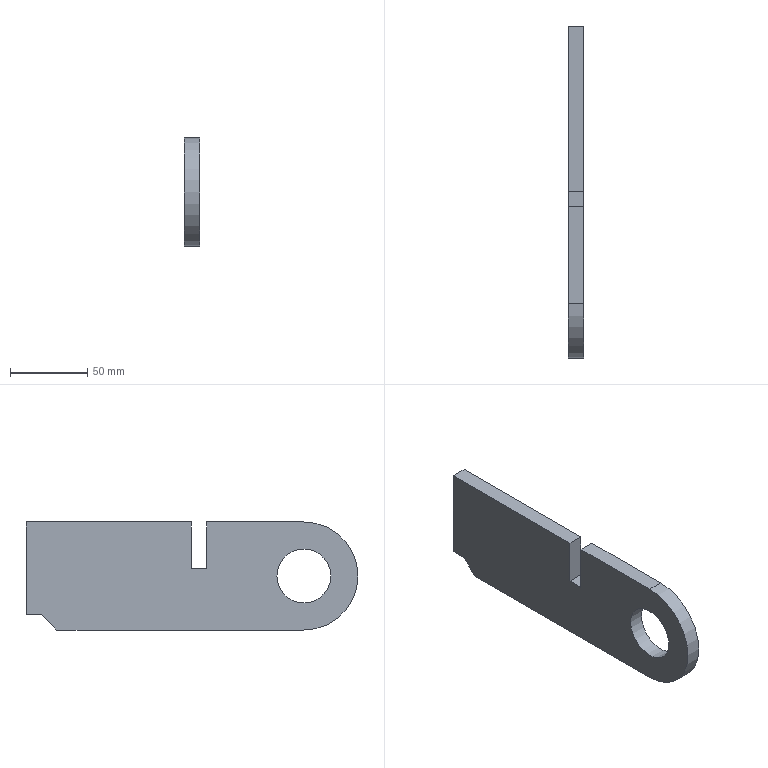Part | STEP file | subframe tilt cylinder mounting plate--000.0
01--20240928 | 1 solid | 13 faces | box 10 x 215 x 70 mm | volume 131121 mm3 | plane 11 | cylinder 2 | commonest cylinder face diameters 35 x1 70 x1
STEP:
#1=CARTESIAN_POINT('',(0.,0.,0.));
#2=DIRECTION('',(0.,0.,1.));
#3=DIRECTION('',(1.,0.,0.));
#4=AXIS2_PLACEMENT_3D('',#1,#2,#3);
#5=CARTESIAN_POINT('',(-630.,216.,-35.));
#6=VERTEX_POINT('',#5);
#7=CARTESIAN_POINT('',(-630.,198.5,-35.));
#8=DIRECTION('',(1.,0.,0.));
#9=DIRECTION('',(0.,1.,0.));
#10=AXIS2_PLACEMENT_3D('',#7,#8,#9);
#11=CIRCLE('',#10,17.5);
#12=CARTESIAN_POINT('',(-630.,-284.,-150.));
#13=DIRECTION('',(1.,0.,0.));
#14=DIRECTION('',(0.,-1.,0.));
#15=AXIS2_PLACEMENT_3D('',#12,#13,#14);
#16=PLANE('',#15);
#17=CARTESIAN_POINT('',(-482.5,-115.));
#18=DIRECTION('',(-1.,0.));
#19=AXIS2_PLACEMENT_2D('',#17,#18);
#20=CIRCLE('',#19,17.5);
#21=(GEOMETRIC_REPRESENTATION_CONTEXT(2)PARAMETRIC_REPRESENTATION_CONTEXT()REPRESENTATION_CONTEXT('',''));
#22=DEFINITIONAL_REPRESENTATION('',(#20),#21);
#23=PCURVE('',#16,#22);
#24=CARTESIAN_POINT('',(-1050.,198.5,-35.));
#25=DIRECTION('',(1.,0.,0.));
#26=DIRECTION('',(0.,0.,1.));
#27=AXIS2_PLACEMENT_3D('',#24,#25,#26);
#28=CYLINDRICAL_SURFACE('',#27,17.5);
#29=CARTESIAN_POINT('',(4.712,420.));
#30=DIRECTION('',(1.,0.));
#31=VECTOR('',#30,1.);
#32=LINE('',#29,#31);
#33=(GEOMETRIC_REPRESENTATION_CONTEXT(2)PARAMETRIC_REPRESENTATION_CONTEXT()REPRESENTATION_CONTEXT('',''));
#34=DEFINITIONAL_REPRESENTATION('',(#32),#33);
#35=PCURVE('',#28,#34);
#36=SURFACE_CURVE('',#11,(#23,#35),.PCURVE_S1.);
#37=EDGE_CURVE('',#6,#6,#36,.T.);
#38=ORIENTED_EDGE('',*,*,#37,.F.);
#39=EDGE_LOOP('',(#38));
#40=FACE_BOUND('',#39,.T.);
#41=CARTESIAN_POINT('',(-630.,198.5,0.));
#42=VERTEX_POINT('',#41);
#43=CARTESIAN_POINT('',(-630.,198.5,-70.));
#44=VERTEX_POINT('',#43);
#45=CARTESIAN_POINT('',(-630.,198.5,-35.));
#46=DIRECTION('',(1.,0.,0.));
#47=DIRECTION('',(0.,1.,0.));
#48=AXIS2_PLACEMENT_3D('',#45,#46,#47);
#49=CIRCLE('',#48,35.);
#50=CARTESIAN_POINT('',(-482.5,-115.));
#51=DIRECTION('',(-1.,0.));
#52=AXIS2_PLACEMENT_2D('',#50,#51);
#53=CIRCLE('',#52,35.);
#54=(GEOMETRIC_REPRESENTATION_CONTEXT(2)PARAMETRIC_REPRESENTATION_CONTEXT()REPRESENTATION_CONTEXT('',''));
#55=DEFINITIONAL_REPRESENTATION('',(#53),#54);
#56=PCURVE('',#16,#55);
#57=CARTESIAN_POINT('',(-700.,198.5,-35.));
#58=DIRECTION('',(-1.,0.,0.));
#59=DIRECTION('',(0.,0.,-1.));
#60=AXIS2_PLACEMENT_3D('',#57,#58,#59);
#61=CYLINDRICAL_SURFACE('',#60,35.);
#62=CARTESIAN_POINT('',(4.712,-70.));
#63=DIRECTION('',(-1.,0.));
#64=VECTOR('',#63,1.);
#65=LINE('',#62,#64);
#66=(GEOMETRIC_REPRESENTATION_CONTEXT(2)PARAMETRIC_REPRESENTATION_CONTEXT()REPRESENTATION_CONTEXT('',''));
#67=DEFINITIONAL_REPRESENTATION('',(#65),#66);
#68=PCURVE('',#61,#67);
#69=SURFACE_CURVE('',#49,(#56,#68),.PCURVE_S1.);
#70=EDGE_CURVE('',#42,#44,#69,.T.);
#71=ORIENTED_EDGE('',*,*,#70,.T.);
#72=CARTESIAN_POINT('',(-630.,358.5,-70.));
#73=VERTEX_POINT('',#72);
#74=CARTESIAN_POINT('',(-630.,198.5,-70.));
#75=DIRECTION('',(0.,-1.,0.));
#76=VECTOR('',#75,1.);
#77=LINE('',#74,#76);
#78=CARTESIAN_POINT('',(-482.5,-80.));
#79=DIRECTION('',(1.,0.));
#80=VECTOR('',#79,1.);
#81=LINE('',#78,#80);
#82=(GEOMETRIC_REPRESENTATION_CONTEXT(2)PARAMETRIC_REPRESENTATION_CONTEXT()REPRESENTATION_CONTEXT('',''));
#83=DEFINITIONAL_REPRESENTATION('',(#81),#82);
#84=PCURVE('',#16,#83);
#85=CARTESIAN_POINT('',(-700.,198.5,-70.));
#86=DIRECTION('',(0.,0.,-1.));
#87=DIRECTION('',(1.,0.,0.));
#88=AXIS2_PLACEMENT_3D('',#85,#86,#87);
#89=PLANE('',#88);
#90=CARTESIAN_POINT('',(70.,0.));
#91=DIRECTION('',(0.,1.));
#92=VECTOR('',#91,1.);
#93=LINE('',#90,#92);
#94=(GEOMETRIC_REPRESENTATION_CONTEXT(2)PARAMETRIC_REPRESENTATION_CONTEXT()REPRESENTATION_CONTEXT('',''));
#95=DEFINITIONAL_REPRESENTATION('',(#93),#94);
#96=PCURVE('',#89,#95);
#97=SURFACE_CURVE('',#77,(#84,#96),.PCURVE_S1.);
#98=EDGE_CURVE('',#73,#44,#97,.T.);
#99=ORIENTED_EDGE('',*,*,#98,.F.);
#100=CARTESIAN_POINT('',(-630.,368.5,-60.));
#101=VERTEX_POINT('',#100);
#102=CARTESIAN_POINT('',(-630.,-2.75,-431.25));
#103=DIRECTION('',(0.,0.7071,0.7071));
#104=VECTOR('',#103,1.);
#105=LINE('',#102,#104);
#106=CARTESIAN_POINT('',(-281.25,281.25));
#107=DIRECTION('',(-0.7071,-0.7071));
#108=VECTOR('',#107,1.);
#109=LINE('',#106,#108);
#110=(GEOMETRIC_REPRESENTATION_CONTEXT(2)PARAMETRIC_REPRESENTATION_CONTEXT()REPRESENTATION_CONTEXT('',''));
#111=DEFINITIONAL_REPRESENTATION('',(#109),#110);
#112=PCURVE('',#16,#111);
#113=CARTESIAN_POINT('',(600.173,368.5,-60.));
#114=DIRECTION('',(0.,-0.7071,0.7071));
#115=DIRECTION('',(1.,0.,0.));
#116=AXIS2_PLACEMENT_3D('',#113,#114,#115);
#117=PLANE('',#116);
#118=CARTESIAN_POINT('',(-1230.173,-525.027));
#119=DIRECTION('',(0.,1.));
#120=VECTOR('',#119,1.);
#121=LINE('',#118,#120);
#122=(GEOMETRIC_REPRESENTATION_CONTEXT(2)PARAMETRIC_REPRESENTATION_CONTEXT()REPRESENTATION_CONTEXT('',''));
#123=DEFINITIONAL_REPRESENTATION('',(#121),#122);
#124=PCURVE('',#117,#123);
#125=SURFACE_CURVE('',#105,(#112,#124),.PCURVE_S1.);
#126=EDGE_CURVE('',#73,#101,#125,.T.);
#127=ORIENTED_EDGE('',*,*,#126,.T.);
#128=CARTESIAN_POINT('',(-630.,378.5,-60.));
#129=VERTEX_POINT('',#128);
#130=CARTESIAN_POINT('',(-630.,-284.,-60.));
#131=DIRECTION('',(0.,1.,0.));
#132=VECTOR('',#131,1.);
#133=LINE('',#130,#132);
#134=CARTESIAN_POINT('',(0.,-90.));
#135=DIRECTION('',(-1.,0.));
#136=VECTOR('',#135,1.);
#137=LINE('',#134,#136);
#138=(GEOMETRIC_REPRESENTATION_CONTEXT(2)PARAMETRIC_REPRESENTATION_CONTEXT()REPRESENTATION_CONTEXT('',''));
#139=DEFINITIONAL_REPRESENTATION('',(#137),#138);
#140=PCURVE('',#16,#139);
#141=CARTESIAN_POINT('',(-635.,288.5,-60.));
#142=DIRECTION('',(0.,0.,-1.));
#143=DIRECTION('',(1.,0.,0.));
#144=AXIS2_PLACEMENT_3D('',#141,#142,#143);
#145=PLANE('',#144);
#146=CARTESIAN_POINT('',(5.,572.5));
#147=DIRECTION('',(0.,-1.));
#148=VECTOR('',#147,1.);
#149=LINE('',#146,#148);
#150=(GEOMETRIC_REPRESENTATION_CONTEXT(2)PARAMETRIC_REPRESENTATION_CONTEXT()REPRESENTATION_CONTEXT('',''));
#151=DEFINITIONAL_REPRESENTATION('',(#149),#150);
#152=PCURVE('',#145,#151);
#153=SURFACE_CURVE('',#133,(#140,#152),.PCURVE_S1.);
#154=EDGE_CURVE('',#101,#129,#153,.T.);
#155=ORIENTED_EDGE('',*,*,#154,.T.);
#156=CARTESIAN_POINT('',(-630.,378.5,0.));
#157=VERTEX_POINT('',#156);
#158=CARTESIAN_POINT('',(-630.,378.5,-20.));
#159=DIRECTION('',(0.,0.,-1.));
#160=VECTOR('',#159,1.);
#161=LINE('',#158,#160);
#162=CARTESIAN_POINT('',(-662.5,-130.));
#163=DIRECTION('',(0.,1.));
#164=VECTOR('',#163,1.);
#165=LINE('',#162,#164);
#166=(GEOMETRIC_REPRESENTATION_CONTEXT(2)PARAMETRIC_REPRESENTATION_CONTEXT()REPRESENTATION_CONTEXT('',''));
#167=DEFINITIONAL_REPRESENTATION('',(#165),#166);
#168=PCURVE('',#16,#167);
#169=CARTESIAN_POINT('',(600.173,378.5,-20.));
#170=DIRECTION('',(0.,1.,0.));
#171=DIRECTION('',(0.9613,0.,0.2756));
#172=AXIS2_PLACEMENT_3D('',#169,#170,#171);
#173=PLANE('',#172);
#174=CARTESIAN_POINT('',(-1182.518,-339.082));
#175=DIRECTION('',(-0.2756,0.9613));
#176=VECTOR('',#175,1.);
#177=LINE('',#174,#176);
#178=(GEOMETRIC_REPRESENTATION_CONTEXT(2)PARAMETRIC_REPRESENTATION_CONTEXT()REPRESENTATION_CONTEXT('',''));
#179=DEFINITIONAL_REPRESENTATION('',(#177),#178);
#180=PCURVE('',#173,#179);
#181=SURFACE_CURVE('',#161,(#168,#180),.PCURVE_S1.);
#182=EDGE_CURVE('',#157,#129,#181,.T.);
#183=ORIENTED_EDGE('',*,*,#182,.F.);
#184=CARTESIAN_POINT('',(-630.,271.5,0.));
#185=VERTEX_POINT('',#184);
#186=CARTESIAN_POINT('',(-630.,-488.,0.));
#187=DIRECTION('',(0.,1.,0.));
#188=VECTOR('',#187,1.);
#189=LINE('',#186,#188);
#190=CARTESIAN_POINT('',(204.,-150.));
#191=DIRECTION('',(-1.,0.));
#192=VECTOR('',#191,1.);
#193=LINE('',#190,#192);
#194=(GEOMETRIC_REPRESENTATION_CONTEXT(2)PARAMETRIC_REPRESENTATION_CONTEXT()REPRESENTATION_CONTEXT('',''));
#195=DEFINITIONAL_REPRESENTATION('',(#193),#194);
#196=PCURVE('',#16,#195);
#197=CARTESIAN_POINT('',(-750.,-488.,0.));
#198=DIRECTION('',(0.,0.,1.));
#199=DIRECTION('',(0.,1.,0.));
#200=AXIS2_PLACEMENT_3D('',#197,#198,#199);
#201=PLANE('',#200);
#202=CARTESIAN_POINT('',(0.,-120.));
#203=DIRECTION('',(1.,0.));
#204=VECTOR('',#203,1.);
#205=LINE('',#202,#204);
#206=(GEOMETRIC_REPRESENTATION_CONTEXT(2)PARAMETRIC_REPRESENTATION_CONTEXT()REPRESENTATION_CONTEXT('',''));
#207=DEFINITIONAL_REPRESENTATION('',(#205),#206);
#208=PCURVE('',#201,#207);
#209=SURFACE_CURVE('',#189,(#196,#208),.PCURVE_S1.);
#210=EDGE_CURVE('',#185,#157,#209,.T.);
#211=ORIENTED_EDGE('',*,*,#210,.F.);
#212=CARTESIAN_POINT('',(-630.,271.5,-30.));
#213=VERTEX_POINT('',#212);
#214=CARTESIAN_POINT('',(-630.,271.5,-150.));
#215=DIRECTION('',(0.,0.,1.));
#216=VECTOR('',#215,1.);
#217=LINE('',#214,#216);
#218=CARTESIAN_POINT('',(-555.5,0.));
#219=DIRECTION('',(0.,-1.));
#220=VECTOR('',#219,1.);
#221=LINE('',#218,#220);
#222=(GEOMETRIC_REPRESENTATION_CONTEXT(2)PARAMETRIC_REPRESENTATION_CONTEXT()REPRESENTATION_CONTEXT('',''));
#223=DEFINITIONAL_REPRESENTATION('',(#221),#222);
#224=PCURVE('',#16,#223);
#225=CARTESIAN_POINT('',(-630.,271.5,-60.));
#226=DIRECTION('',(0.,1.,0.));
#227=DIRECTION('',(0.,0.,-1.));
#228=AXIS2_PLACEMENT_3D('',#225,#226,#227);
#229=PLANE('',#228);
#230=CARTESIAN_POINT('',(90.,0.));
#231=DIRECTION('',(-1.,0.));
#232=VECTOR('',#231,1.);
#233=LINE('',#230,#232);
#234=(GEOMETRIC_REPRESENTATION_CONTEXT(2)PARAMETRIC_REPRESENTATION_CONTEXT()REPRESENTATION_CONTEXT('',''));
#235=DEFINITIONAL_REPRESENTATION('',(#233),#234);
#236=PCURVE('',#229,#235);
#237=SURFACE_CURVE('',#217,(#224,#236),.PCURVE_S1.);
#238=EDGE_CURVE('',#213,#185,#237,.T.);
#239=ORIENTED_EDGE('',*,*,#238,.F.);
#240=CARTESIAN_POINT('',(-630.,261.5,-30.));
#241=VERTEX_POINT('',#240);
#242=CARTESIAN_POINT('',(-630.,266.5,-30.));
#243=DIRECTION('',(0.,1.,0.));
#244=VECTOR('',#243,1.);
#245=LINE('',#242,#244);
#246=CARTESIAN_POINT('',(-550.5,-120.));
#247=DIRECTION('',(-1.,0.));
#248=VECTOR('',#247,1.);
#249=LINE('',#246,#248);
#250=(GEOMETRIC_REPRESENTATION_CONTEXT(2)PARAMETRIC_REPRESENTATION_CONTEXT()REPRESENTATION_CONTEXT('',''));
#251=DEFINITIONAL_REPRESENTATION('',(#249),#250);
#252=PCURVE('',#16,#251);
#253=CARTESIAN_POINT('',(-625.,266.5,-30.));
#254=DIRECTION('',(0.,0.,1.));
#255=DIRECTION('',(-1.,0.,0.));
#256=AXIS2_PLACEMENT_3D('',#253,#254,#255);
#257=PLANE('',#256);
#258=CARTESIAN_POINT('',(5.,0.));
#259=DIRECTION('',(0.,-1.));
#260=VECTOR('',#259,1.);
#261=LINE('',#258,#260);
#262=(GEOMETRIC_REPRESENTATION_CONTEXT(2)PARAMETRIC_REPRESENTATION_CONTEXT()REPRESENTATION_CONTEXT('',''));
#263=DEFINITIONAL_REPRESENTATION('',(#261),#262);
#264=PCURVE('',#257,#263);
#265=SURFACE_CURVE('',#245,(#252,#264),.PCURVE_S1.);
#266=EDGE_CURVE('',#241,#213,#265,.T.);
#267=ORIENTED_EDGE('',*,*,#266,.F.);
#268=CARTESIAN_POINT('',(-630.,261.5,0.));
#269=VERTEX_POINT('',#268);
#270=CARTESIAN_POINT('',(-630.,261.5,-150.));
#271=DIRECTION('',(0.,0.,-1.));
#272=VECTOR('',#271,1.);
#273=LINE('',#270,#272);
#274=CARTESIAN_POINT('',(-545.5,0.));
#275=DIRECTION('',(0.,1.));
#276=VECTOR('',#275,1.);
#277=LINE('',#274,#276);
#278=(GEOMETRIC_REPRESENTATION_CONTEXT(2)PARAMETRIC_REPRESENTATION_CONTEXT()REPRESENTATION_CONTEXT('',''));
#279=DEFINITIONAL_REPRESENTATION('',(#277),#278);
#280=PCURVE('',#16,#279);
#281=CARTESIAN_POINT('',(-630.,261.5,-60.));
#282=DIRECTION('',(0.,1.,0.));
#283=DIRECTION('',(0.,0.,-1.));
#284=AXIS2_PLACEMENT_3D('',#281,#282,#283);
#285=PLANE('',#284);
#286=CARTESIAN_POINT('',(90.,0.));
#287=DIRECTION('',(1.,0.));
#288=VECTOR('',#287,1.);
#289=LINE('',#286,#288);
#290=(GEOMETRIC_REPRESENTATION_CONTEXT(2)PARAMETRIC_REPRESENTATION_CONTEXT()REPRESENTATION_CONTEXT('',''));
#291=DEFINITIONAL_REPRESENTATION('',(#289),#290);
#292=PCURVE('',#285,#291);
#293=SURFACE_CURVE('',#273,(#280,#292),.PCURVE_S1.);
#294=EDGE_CURVE('',#269,#241,#293,.T.);
#295=ORIENTED_EDGE('',*,*,#294,.F.);
#296=CARTESIAN_POINT('',(-630.,-488.,0.));
#297=DIRECTION('',(0.,1.,0.));
#298=VECTOR('',#297,1.);
#299=LINE('',#296,#298);
#300=CARTESIAN_POINT('',(204.,-150.));
#301=DIRECTION('',(-1.,0.));
#302=VECTOR('',#301,1.);
#303=LINE('',#300,#302);
#304=(GEOMETRIC_REPRESENTATION_CONTEXT(2)PARAMETRIC_REPRESENTATION_CONTEXT()REPRESENTATION_CONTEXT('',''));
#305=DEFINITIONAL_REPRESENTATION('',(#303),#304);
#306=PCURVE('',#16,#305);
#307=CARTESIAN_POINT('',(-750.,-488.,0.));
#308=DIRECTION('',(0.,0.,1.));
#309=DIRECTION('',(0.,1.,0.));
#310=AXIS2_PLACEMENT_3D('',#307,#308,#309);
#311=PLANE('',#310);
#312=CARTESIAN_POINT('',(0.,-120.));
#313=DIRECTION('',(1.,0.));
#314=VECTOR('',#313,1.);
#315=LINE('',#312,#314);
#316=(GEOMETRIC_REPRESENTATION_CONTEXT(2)PARAMETRIC_REPRESENTATION_CONTEXT()REPRESENTATION_CONTEXT('',''));
#317=DEFINITIONAL_REPRESENTATION('',(#315),#316);
#318=PCURVE('',#311,#317);
#319=SURFACE_CURVE('',#299,(#306,#318),.PCURVE_S1.);
#320=EDGE_CURVE('',#42,#269,#319,.T.);
#321=ORIENTED_EDGE('',*,*,#320,.F.);
#322=EDGE_LOOP('',(#71,#99,#127,#155,#183,#211,#239,#267,#295,#321));
#323=FACE_BOUND('',#322,.T.);
#324=ADVANCED_FACE('',(#40,#323),#16,.T.);
#325=CARTESIAN_POINT('',(-640.,181.,-35.));
#326=VERTEX_POINT('',#325);
#327=CARTESIAN_POINT('',(-640.,216.,-35.));
#328=VERTEX_POINT('',#327);
#329=CARTESIAN_POINT('',(-640.,198.5,-35.));
#330=DIRECTION('',(-1.,0.,0.));
#331=DIRECTION('',(0.,-1.,0.));
#332=AXIS2_PLACEMENT_3D('',#329,#330,#331);
#333=CIRCLE('',#332,17.5);
#334=CARTESIAN_POINT('',(-640.,-284.,-150.));
#335=DIRECTION('',(-1.,0.,0.));
#336=DIRECTION('',(0.,1.,0.));
#337=AXIS2_PLACEMENT_3D('',#334,#335,#336);
#338=PLANE('',#337);
#339=CARTESIAN_POINT('',(482.5,-115.));
#340=DIRECTION('',(-1.,0.));
#341=AXIS2_PLACEMENT_2D('',#339,#340);
#342=CIRCLE('',#341,17.5);
#343=(GEOMETRIC_REPRESENTATION_CONTEXT(2)PARAMETRIC_REPRESENTATION_CONTEXT()REPRESENTATION_CONTEXT('',''));
#344=DEFINITIONAL_REPRESENTATION('',(#342),#343);
#345=PCURVE('',#338,#344);
#346=CARTESIAN_POINT('',(7.854,410.));
#347=DIRECTION('',(-1.,0.));
#348=VECTOR('',#347,1.);
#349=LINE('',#346,#348);
#350=(GEOMETRIC_REPRESENTATION_CONTEXT(2)PARAMETRIC_REPRESENTATION_CONTEXT()REPRESENTATION_CONTEXT('',''));
#351=DEFINITIONAL_REPRESENTATION('',(#349),#350);
#352=PCURVE('',#28,#351);
#353=SURFACE_CURVE('',#333,(#345,#352),.PCURVE_S1.);
#354=EDGE_CURVE('',#326,#328,#353,.T.);
#355=ORIENTED_EDGE('',*,*,#354,.F.);
#356=CARTESIAN_POINT('',(-640.,198.5,-35.));
#357=DIRECTION('',(-1.,0.,0.));
#358=DIRECTION('',(0.,-1.,0.));
#359=AXIS2_PLACEMENT_3D('',#356,#357,#358);
#360=CIRCLE('',#359,17.5);
#361=CARTESIAN_POINT('',(482.5,-115.));
#362=DIRECTION('',(-1.,0.));
#363=AXIS2_PLACEMENT_2D('',#361,#362);
#364=CIRCLE('',#363,17.5);
#365=(GEOMETRIC_REPRESENTATION_CONTEXT(2)PARAMETRIC_REPRESENTATION_CONTEXT()REPRESENTATION_CONTEXT('',''));
#366=DEFINITIONAL_REPRESENTATION('',(#364),#365);
#367=PCURVE('',#338,#366);
#368=CARTESIAN_POINT('',(14.137,410.));
#369=DIRECTION('',(-1.,0.));
#370=VECTOR('',#369,1.);
#371=LINE('',#368,#370);
#372=(GEOMETRIC_REPRESENTATION_CONTEXT(2)PARAMETRIC_REPRESENTATION_CONTEXT()REPRESENTATION_CONTEXT('',''));
#373=DEFINITIONAL_REPRESENTATION('',(#371),#372);
#374=PCURVE('',#28,#373);
#375=SURFACE_CURVE('',#360,(#367,#374),.PCURVE_S1.);
#376=EDGE_CURVE('',#328,#326,#375,.T.);
#377=ORIENTED_EDGE('',*,*,#376,.F.);
#378=EDGE_LOOP('',(#355,#377));
#379=FACE_BOUND('',#378,.T.);
#380=CARTESIAN_POINT('',(-640.,378.5,-60.));
#381=VERTEX_POINT('',#380);
#382=CARTESIAN_POINT('',(-640.,378.5,0.));
#383=VERTEX_POINT('',#382);
#384=CARTESIAN_POINT('',(-640.,378.5,-20.));
#385=DIRECTION('',(0.,0.,1.));
#386=VECTOR('',#385,1.);
#387=LINE('',#384,#386);
#388=CARTESIAN_POINT('',(662.5,-130.));
#389=DIRECTION('',(0.,-1.));
#390=VECTOR('',#389,1.);
#391=LINE('',#388,#390);
#392=(GEOMETRIC_REPRESENTATION_CONTEXT(2)PARAMETRIC_REPRESENTATION_CONTEXT()REPRESENTATION_CONTEXT('',''));
#393=DEFINITIONAL_REPRESENTATION('',(#391),#392);
#394=PCURVE('',#338,#393);
#395=CARTESIAN_POINT('',(-1192.131,-341.838));
#396=DIRECTION('',(0.2756,-0.9613));
#397=VECTOR('',#396,1.);
#398=LINE('',#395,#397);
#399=(GEOMETRIC_REPRESENTATION_CONTEXT(2)PARAMETRIC_REPRESENTATION_CONTEXT()REPRESENTATION_CONTEXT('',''));
#400=DEFINITIONAL_REPRESENTATION('',(#398),#399);
#401=PCURVE('',#173,#400);
#402=SURFACE_CURVE('',#387,(#394,#401),.PCURVE_S1.);
#403=EDGE_CURVE('',#381,#383,#402,.T.);
#404=ORIENTED_EDGE('',*,*,#403,.F.);
#405=CARTESIAN_POINT('',(-640.,368.5,-60.));
#406=VERTEX_POINT('',#405);
#407=CARTESIAN_POINT('',(-640.,-284.,-60.));
#408=DIRECTION('',(0.,-1.,0.));
#409=VECTOR('',#408,1.);
#410=LINE('',#407,#409);
#411=CARTESIAN_POINT('',(0.,-90.));
#412=DIRECTION('',(-1.,0.));
#413=VECTOR('',#412,1.);
#414=LINE('',#411,#413);
#415=(GEOMETRIC_REPRESENTATION_CONTEXT(2)PARAMETRIC_REPRESENTATION_CONTEXT()REPRESENTATION_CONTEXT('',''));
#416=DEFINITIONAL_REPRESENTATION('',(#414),#415);
#417=PCURVE('',#338,#416);
#418=CARTESIAN_POINT('',(-5.,572.5));
#419=DIRECTION('',(0.,1.));
#420=VECTOR('',#419,1.);
#421=LINE('',#418,#420);
#422=(GEOMETRIC_REPRESENTATION_CONTEXT(2)PARAMETRIC_REPRESENTATION_CONTEXT()REPRESENTATION_CONTEXT('',''));
#423=DEFINITIONAL_REPRESENTATION('',(#421),#422);
#424=PCURVE('',#145,#423);
#425=SURFACE_CURVE('',#410,(#417,#424),.PCURVE_S1.);
#426=EDGE_CURVE('',#381,#406,#425,.T.);
#427=ORIENTED_EDGE('',*,*,#426,.T.);
#428=CARTESIAN_POINT('',(-640.,358.5,-70.));
#429=VERTEX_POINT('',#428);
#430=CARTESIAN_POINT('',(-640.,-2.75,-431.25));
#431=DIRECTION('',(0.,-0.7071,-0.7071));
#432=VECTOR('',#431,1.);
#433=LINE('',#430,#432);
#434=CARTESIAN_POINT('',(281.25,281.25));
#435=DIRECTION('',(-0.7071,0.7071));
#436=VECTOR('',#435,1.);
#437=LINE('',#434,#436);
#438=(GEOMETRIC_REPRESENTATION_CONTEXT(2)PARAMETRIC_REPRESENTATION_CONTEXT()REPRESENTATION_CONTEXT('',''));
#439=DEFINITIONAL_REPRESENTATION('',(#437),#438);
#440=PCURVE('',#338,#439);
#441=CARTESIAN_POINT('',(-1240.173,-525.027));
#442=DIRECTION('',(0.,-1.));
#443=VECTOR('',#442,1.);
#444=LINE('',#441,#443);
#445=(GEOMETRIC_REPRESENTATION_CONTEXT(2)PARAMETRIC_REPRESENTATION_CONTEXT()REPRESENTATION_CONTEXT('',''));
#446=DEFINITIONAL_REPRESENTATION('',(#444),#445);
#447=PCURVE('',#117,#446);
#448=SURFACE_CURVE('',#433,(#440,#447),.PCURVE_S1.);
#449=EDGE_CURVE('',#406,#429,#448,.T.);
#450=ORIENTED_EDGE('',*,*,#449,.T.);
#451=CARTESIAN_POINT('',(-640.,198.5,-70.));
#452=VERTEX_POINT('',#451);
#453=CARTESIAN_POINT('',(-640.,198.5,-70.));
#454=DIRECTION('',(0.,1.,0.));
#455=VECTOR('',#454,1.);
#456=LINE('',#453,#455);
#457=CARTESIAN_POINT('',(482.5,-80.));
#458=DIRECTION('',(1.,0.));
#459=VECTOR('',#458,1.);
#460=LINE('',#457,#459);
#461=(GEOMETRIC_REPRESENTATION_CONTEXT(2)PARAMETRIC_REPRESENTATION_CONTEXT()REPRESENTATION_CONTEXT('',''));
#462=DEFINITIONAL_REPRESENTATION('',(#460),#461);
#463=PCURVE('',#338,#462);
#464=CARTESIAN_POINT('',(60.,0.));
#465=DIRECTION('',(0.,-1.));
#466=VECTOR('',#465,1.);
#467=LINE('',#464,#466);
#468=(GEOMETRIC_REPRESENTATION_CONTEXT(2)PARAMETRIC_REPRESENTATION_CONTEXT()REPRESENTATION_CONTEXT('',''));
#469=DEFINITIONAL_REPRESENTATION('',(#467),#468);
#470=PCURVE('',#89,#469);
#471=SURFACE_CURVE('',#456,(#463,#470),.PCURVE_S1.);
#472=EDGE_CURVE('',#452,#429,#471,.T.);
#473=ORIENTED_EDGE('',*,*,#472,.F.);
#474=CARTESIAN_POINT('',(-640.,198.5,0.));
#475=VERTEX_POINT('',#474);
#476=CARTESIAN_POINT('',(-640.,198.5,-35.));
#477=DIRECTION('',(-1.,0.,0.));
#478=DIRECTION('',(0.,-1.,0.));
#479=AXIS2_PLACEMENT_3D('',#476,#477,#478);
#480=CIRCLE('',#479,35.);
#481=CARTESIAN_POINT('',(482.5,-115.));
#482=DIRECTION('',(-1.,0.));
#483=AXIS2_PLACEMENT_2D('',#481,#482);
#484=CIRCLE('',#483,35.);
#485=(GEOMETRIC_REPRESENTATION_CONTEXT(2)PARAMETRIC_REPRESENTATION_CONTEXT()REPRESENTATION_CONTEXT('',''));
#486=DEFINITIONAL_REPRESENTATION('',(#484),#485);
#487=PCURVE('',#338,#486);
#488=CARTESIAN_POINT('',(-4.712,-60.));
#489=DIRECTION('',(1.,0.));
#490=VECTOR('',#489,1.);
#491=LINE('',#488,#490);
#492=(GEOMETRIC_REPRESENTATION_CONTEXT(2)PARAMETRIC_REPRESENTATION_CONTEXT()REPRESENTATION_CONTEXT('',''));
#493=DEFINITIONAL_REPRESENTATION('',(#491),#492);
#494=PCURVE('',#61,#493);
#495=SURFACE_CURVE('',#480,(#487,#494),.PCURVE_S1.);
#496=EDGE_CURVE('',#452,#475,#495,.T.);
#497=ORIENTED_EDGE('',*,*,#496,.T.);
#498=CARTESIAN_POINT('',(-640.,261.5,0.));
#499=VERTEX_POINT('',#498);
#500=CARTESIAN_POINT('',(-640.,-488.,0.));
#501=DIRECTION('',(0.,-1.,0.));
#502=VECTOR('',#501,1.);
#503=LINE('',#500,#502);
#504=CARTESIAN_POINT('',(-204.,-150.));
#505=DIRECTION('',(-1.,0.));
#506=VECTOR('',#505,1.);
#507=LINE('',#504,#506);
#508=(GEOMETRIC_REPRESENTATION_CONTEXT(2)PARAMETRIC_REPRESENTATION_CONTEXT()REPRESENTATION_CONTEXT('',''));
#509=DEFINITIONAL_REPRESENTATION('',(#507),#508);
#510=PCURVE('',#338,#509);
#511=CARTESIAN_POINT('',(0.,-110.));
#512=DIRECTION('',(-1.,0.));
#513=VECTOR('',#512,1.);
#514=LINE('',#511,#513);
#515=(GEOMETRIC_REPRESENTATION_CONTEXT(2)PARAMETRIC_REPRESENTATION_CONTEXT()REPRESENTATION_CONTEXT('',''));
#516=DEFINITIONAL_REPRESENTATION('',(#514),#515);
#517=PCURVE('',#311,#516);
#518=SURFACE_CURVE('',#503,(#510,#517),.PCURVE_S1.);
#519=EDGE_CURVE('',#499,#475,#518,.T.);
#520=ORIENTED_EDGE('',*,*,#519,.F.);
#521=CARTESIAN_POINT('',(-640.,261.5,-30.));
#522=VERTEX_POINT('',#521);
#523=CARTESIAN_POINT('',(-640.,261.5,-150.));
#524=DIRECTION('',(0.,0.,1.));
#525=VECTOR('',#524,1.);
#526=LINE('',#523,#525);
#527=CARTESIAN_POINT('',(545.5,0.));
#528=DIRECTION('',(0.,-1.));
#529=VECTOR('',#528,1.);
#530=LINE('',#527,#529);
#531=(GEOMETRIC_REPRESENTATION_CONTEXT(2)PARAMETRIC_REPRESENTATION_CONTEXT()REPRESENTATION_CONTEXT('',''));
#532=DEFINITIONAL_REPRESENTATION('',(#530),#531);
#533=PCURVE('',#338,#532);
#534=CARTESIAN_POINT('',(90.,10.));
#535=DIRECTION('',(-1.,0.));
#536=VECTOR('',#535,1.);
#537=LINE('',#534,#536);
#538=(GEOMETRIC_REPRESENTATION_CONTEXT(2)PARAMETRIC_REPRESENTATION_CONTEXT()REPRESENTATION_CONTEXT('',''));
#539=DEFINITIONAL_REPRESENTATION('',(#537),#538);
#540=PCURVE('',#285,#539);
#541=SURFACE_CURVE('',#526,(#533,#540),.PCURVE_S1.);
#542=EDGE_CURVE('',#522,#499,#541,.T.);
#543=ORIENTED_EDGE('',*,*,#542,.F.);
#544=CARTESIAN_POINT('',(-640.,271.5,-30.));
#545=VERTEX_POINT('',#544);
#546=CARTESIAN_POINT('',(-640.,266.5,-30.));
#547=DIRECTION('',(0.,-1.,0.));
#548=VECTOR('',#547,1.);
#549=LINE('',#546,#548);
#550=CARTESIAN_POINT('',(550.5,-120.));
#551=DIRECTION('',(-1.,0.));
#552=VECTOR('',#551,1.);
#553=LINE('',#550,#552);
#554=(GEOMETRIC_REPRESENTATION_CONTEXT(2)PARAMETRIC_REPRESENTATION_CONTEXT()REPRESENTATION_CONTEXT('',''));
#555=DEFINITIONAL_REPRESENTATION('',(#553),#554);
#556=PCURVE('',#338,#555);
#557=CARTESIAN_POINT('',(15.,0.));
#558=DIRECTION('',(0.,1.));
#559=VECTOR('',#558,1.);
#560=LINE('',#557,#559);
#561=(GEOMETRIC_REPRESENTATION_CONTEXT(2)PARAMETRIC_REPRESENTATION_CONTEXT()REPRESENTATION_CONTEXT('',''));
#562=DEFINITIONAL_REPRESENTATION('',(#560),#561);
#563=PCURVE('',#257,#562);
#564=SURFACE_CURVE('',#549,(#556,#563),.PCURVE_S1.);
#565=EDGE_CURVE('',#545,#522,#564,.T.);
#566=ORIENTED_EDGE('',*,*,#565,.F.);
#567=CARTESIAN_POINT('',(-640.,271.5,0.));
#568=VERTEX_POINT('',#567);
#569=CARTESIAN_POINT('',(-640.,271.5,-150.));
#570=DIRECTION('',(0.,0.,-1.));
#571=VECTOR('',#570,1.);
#572=LINE('',#569,#571);
#573=CARTESIAN_POINT('',(555.5,0.));
#574=DIRECTION('',(0.,1.));
#575=VECTOR('',#574,1.);
#576=LINE('',#573,#575);
#577=(GEOMETRIC_REPRESENTATION_CONTEXT(2)PARAMETRIC_REPRESENTATION_CONTEXT()REPRESENTATION_CONTEXT('',''));
#578=DEFINITIONAL_REPRESENTATION('',(#576),#577);
#579=PCURVE('',#338,#578);
#580=CARTESIAN_POINT('',(90.,10.));
#581=DIRECTION('',(1.,0.));
#582=VECTOR('',#581,1.);
#583=LINE('',#580,#582);
#584=(GEOMETRIC_REPRESENTATION_CONTEXT(2)PARAMETRIC_REPRESENTATION_CONTEXT()REPRESENTATION_CONTEXT('',''));
#585=DEFINITIONAL_REPRESENTATION('',(#583),#584);
#586=PCURVE('',#229,#585);
#587=SURFACE_CURVE('',#572,(#579,#586),.PCURVE_S1.);
#588=EDGE_CURVE('',#568,#545,#587,.T.);
#589=ORIENTED_EDGE('',*,*,#588,.F.);
#590=CARTESIAN_POINT('',(-640.,-488.,0.));
#591=DIRECTION('',(0.,-1.,0.));
#592=VECTOR('',#591,1.);
#593=LINE('',#590,#592);
#594=CARTESIAN_POINT('',(-204.,-150.));
#595=DIRECTION('',(-1.,0.));
#596=VECTOR('',#595,1.);
#597=LINE('',#594,#596);
#598=(GEOMETRIC_REPRESENTATION_CONTEXT(2)PARAMETRIC_REPRESENTATION_CONTEXT()REPRESENTATION_CONTEXT('',''));
#599=DEFINITIONAL_REPRESENTATION('',(#597),#598);
#600=PCURVE('',#338,#599);
#601=CARTESIAN_POINT('',(0.,-110.));
#602=DIRECTION('',(-1.,0.));
#603=VECTOR('',#602,1.);
#604=LINE('',#601,#603);
#605=(GEOMETRIC_REPRESENTATION_CONTEXT(2)PARAMETRIC_REPRESENTATION_CONTEXT()REPRESENTATION_CONTEXT('',''));
#606=DEFINITIONAL_REPRESENTATION('',(#604),#605);
#607=PCURVE('',#201,#606);
#608=SURFACE_CURVE('',#593,(#600,#607),.PCURVE_S1.);
#609=EDGE_CURVE('',#383,#568,#608,.T.);
#610=ORIENTED_EDGE('',*,*,#609,.F.);
#611=EDGE_LOOP('',(#404,#427,#450,#473,#497,#520,#543,#566,#589,#610));
#612=FACE_BOUND('',#611,.T.);
#613=ADVANCED_FACE('',(#379,#612),#338,.T.);
#614=ORIENTED_EDGE('',*,*,#182,.T.);
#615=CARTESIAN_POINT('',(600.173,378.5,-60.));
#616=DIRECTION('',(-1.,0.,0.));
#617=VECTOR('',#616,1.);
#618=LINE('',#615,#617);
#619=CARTESIAN_POINT('',(-11.025,38.45));
#620=DIRECTION('',(-0.9613,-0.2756));
#621=VECTOR('',#620,1.);
#622=LINE('',#619,#621);
#623=(GEOMETRIC_REPRESENTATION_CONTEXT(2)PARAMETRIC_REPRESENTATION_CONTEXT()REPRESENTATION_CONTEXT('',''));
#624=DEFINITIONAL_REPRESENTATION('',(#622),#623);
#625=PCURVE('',#173,#624);
#626=CARTESIAN_POINT('',(1235.173,-90.));
#627=DIRECTION('',(-1.,0.));
#628=VECTOR('',#627,1.);
#629=LINE('',#626,#628);
#630=(GEOMETRIC_REPRESENTATION_CONTEXT(2)PARAMETRIC_REPRESENTATION_CONTEXT()REPRESENTATION_CONTEXT('',''));
#631=DEFINITIONAL_REPRESENTATION('',(#629),#630);
#632=PCURVE('',#145,#631);
#633=SURFACE_CURVE('',#618,(#625,#632),.PCURVE_S1.);
#634=EDGE_CURVE('',#129,#381,#633,.T.);
#635=ORIENTED_EDGE('',*,*,#634,.T.);
#636=ORIENTED_EDGE('',*,*,#403,.T.);
#637=CARTESIAN_POINT('',(600.173,378.5,0.));
#638=DIRECTION('',(1.,0.,0.));
#639=VECTOR('',#638,1.);
#640=LINE('',#637,#639);
#641=CARTESIAN_POINT('',(5.513,-19.225));
#642=DIRECTION('',(0.9613,0.2756));
#643=VECTOR('',#642,1.);
#644=LINE('',#641,#643);
#645=(GEOMETRIC_REPRESENTATION_CONTEXT(2)PARAMETRIC_REPRESENTATION_CONTEXT()REPRESENTATION_CONTEXT('',''));
#646=DEFINITIONAL_REPRESENTATION('',(#644),#645);
#647=PCURVE('',#173,#646);
#648=CARTESIAN_POINT('',(866.5,-1350.173));
#649=DIRECTION('',(0.,-1.));
#650=VECTOR('',#649,1.);
#651=LINE('',#648,#650);
#652=(GEOMETRIC_REPRESENTATION_CONTEXT(2)PARAMETRIC_REPRESENTATION_CONTEXT()REPRESENTATION_CONTEXT('',''));
#653=DEFINITIONAL_REPRESENTATION('',(#651),#652);
#654=PCURVE('',#201,#653);
#655=SURFACE_CURVE('',#640,(#647,#654),.PCURVE_S1.);
#656=EDGE_CURVE('',#383,#157,#655,.T.);
#657=ORIENTED_EDGE('',*,*,#656,.T.);
#658=EDGE_LOOP('',(#614,#635,#636,#657));
#659=FACE_BOUND('',#658,.T.);
#660=ADVANCED_FACE('',(#659),#173,.T.);
#661=ORIENTED_EDGE('',*,*,#496,.F.);
#662=CARTESIAN_POINT('',(-700.,198.5,-70.));
#663=DIRECTION('',(-1.,0.,0.));
#664=VECTOR('',#663,1.);
#665=LINE('',#662,#664);
#666=CARTESIAN_POINT('',(0.,0.));
#667=DIRECTION('',(0.,1.));
#668=VECTOR('',#667,1.);
#669=LINE('',#666,#668);
#670=(GEOMETRIC_REPRESENTATION_CONTEXT(2)PARAMETRIC_REPRESENTATION_CONTEXT()REPRESENTATION_CONTEXT('',''));
#671=DEFINITIONAL_REPRESENTATION('',(#669),#670);
#672=PCURVE('',#61,#671);
#673=CARTESIAN_POINT('',(0.,0.));
#674=DIRECTION('',(-1.,0.));
#675=VECTOR('',#674,1.);
#676=LINE('',#673,#675);
#677=(GEOMETRIC_REPRESENTATION_CONTEXT(2)PARAMETRIC_REPRESENTATION_CONTEXT()REPRESENTATION_CONTEXT('',''));
#678=DEFINITIONAL_REPRESENTATION('',(#676),#677);
#679=PCURVE('',#89,#678);
#680=SURFACE_CURVE('',#665,(#672,#679),.PCURVE_S1.);
#681=EDGE_CURVE('',#44,#452,#680,.T.);
#682=ORIENTED_EDGE('',*,*,#681,.F.);
#683=ORIENTED_EDGE('',*,*,#70,.F.);
#684=CARTESIAN_POINT('',(-750.,198.5,0.));
#685=DIRECTION('',(1.,0.,0.));
#686=VECTOR('',#685,1.);
#687=LINE('',#684,#686);
#688=CARTESIAN_POINT('',(3.142,50.));
#689=DIRECTION('',(0.,-1.));
#690=VECTOR('',#689,1.);
#691=LINE('',#688,#690);
#692=(GEOMETRIC_REPRESENTATION_CONTEXT(2)PARAMETRIC_REPRESENTATION_CONTEXT()REPRESENTATION_CONTEXT('',''));
#693=DEFINITIONAL_REPRESENTATION('',(#691),#692);
#694=PCURVE('',#61,#693);
#695=CARTESIAN_POINT('',(686.5,0.));
#696=DIRECTION('',(0.,-1.));
#697=VECTOR('',#696,1.);
#698=LINE('',#695,#697);
#699=(GEOMETRIC_REPRESENTATION_CONTEXT(2)PARAMETRIC_REPRESENTATION_CONTEXT()REPRESENTATION_CONTEXT('',''));
#700=DEFINITIONAL_REPRESENTATION('',(#698),#699);
#701=PCURVE('',#311,#700);
#702=SURFACE_CURVE('',#687,(#694,#701),.PCURVE_S1.);
#703=EDGE_CURVE('',#475,#42,#702,.T.);
#704=ORIENTED_EDGE('',*,*,#703,.F.);
#705=EDGE_LOOP('',(#661,#682,#683,#704));
#706=FACE_BOUND('',#705,.T.);
#707=ADVANCED_FACE('',(#706),#61,.T.);
#708=ORIENTED_EDGE('',*,*,#320,.T.);
#709=CARTESIAN_POINT('',(-630.,261.5,0.));
#710=DIRECTION('',(-1.,0.,0.));
#711=VECTOR('',#710,1.);
#712=LINE('',#709,#711);
#713=CARTESIAN_POINT('',(749.5,-120.));
#714=DIRECTION('',(0.,1.));
#715=VECTOR('',#714,1.);
#716=LINE('',#713,#715);
#717=(GEOMETRIC_REPRESENTATION_CONTEXT(2)PARAMETRIC_REPRESENTATION_CONTEXT()REPRESENTATION_CONTEXT('',''));
#718=DEFINITIONAL_REPRESENTATION('',(#716),#717);
#719=PCURVE('',#311,#718);
#720=CARTESIAN_POINT('',(-60.,0.));
#721=DIRECTION('',(0.,1.));
#722=VECTOR('',#721,1.);
#723=LINE('',#720,#722);
#724=(GEOMETRIC_REPRESENTATION_CONTEXT(2)PARAMETRIC_REPRESENTATION_CONTEXT()REPRESENTATION_CONTEXT('',''));
#725=DEFINITIONAL_REPRESENTATION('',(#723),#724);
#726=PCURVE('',#285,#725);
#727=SURFACE_CURVE('',#712,(#719,#726),.PCURVE_S1.);
#728=EDGE_CURVE('',#269,#499,#727,.T.);
#729=ORIENTED_EDGE('',*,*,#728,.T.);
#730=ORIENTED_EDGE('',*,*,#519,.T.);
#731=ORIENTED_EDGE('',*,*,#703,.T.);
#732=EDGE_LOOP('',(#708,#729,#730,#731));
#733=FACE_BOUND('',#732,.T.);
#734=ADVANCED_FACE('',(#733),#311,.T.);
#735=CARTESIAN_POINT('',(-630.,271.5,0.));
#736=DIRECTION('',(-1.,0.,0.));
#737=VECTOR('',#736,1.);
#738=LINE('',#735,#737);
#739=CARTESIAN_POINT('',(759.5,-120.));
#740=DIRECTION('',(0.,1.));
#741=VECTOR('',#740,1.);
#742=LINE('',#739,#741);
#743=(GEOMETRIC_REPRESENTATION_CONTEXT(2)PARAMETRIC_REPRESENTATION_CONTEXT()REPRESENTATION_CONTEXT('',''));
#744=DEFINITIONAL_REPRESENTATION('',(#742),#743);
#745=PCURVE('',#201,#744);
#746=CARTESIAN_POINT('',(-60.,0.));
#747=DIRECTION('',(0.,1.));
#748=VECTOR('',#747,1.);
#749=LINE('',#746,#748);
#750=(GEOMETRIC_REPRESENTATION_CONTEXT(2)PARAMETRIC_REPRESENTATION_CONTEXT()REPRESENTATION_CONTEXT('',''));
#751=DEFINITIONAL_REPRESENTATION('',(#749),#750);
#752=PCURVE('',#229,#751);
#753=SURFACE_CURVE('',#738,(#745,#752),.PCURVE_S1.);
#754=EDGE_CURVE('',#185,#568,#753,.T.);
#755=ORIENTED_EDGE('',*,*,#754,.F.);
#756=ORIENTED_EDGE('',*,*,#210,.T.);
#757=ORIENTED_EDGE('',*,*,#656,.F.);
#758=ORIENTED_EDGE('',*,*,#609,.T.);
#759=EDGE_LOOP('',(#755,#756,#757,#758));
#760=FACE_BOUND('',#759,.T.);
#761=ADVANCED_FACE('',(#760),#201,.T.);
#762=ORIENTED_EDGE('',*,*,#376,.F.);
#763=CARTESIAN_POINT('',(-640.,216.,-35.));
#764=CARTESIAN_POINT('',(-630.,216.,-35.));
#765=B_SPLINE_CURVE_WITH_KNOTS('',1,(#763,#764),.UNSPECIFIED.,.F.,.F.,(2,2),(410.,420.),.PIECEWISE_BEZIER_KNOTS.);
#766=CARTESIAN_POINT('',(10.996,0.));
#767=DIRECTION('',(0.,1.));
#768=VECTOR('',#767,1.);
#769=LINE('',#766,#768);
#770=(GEOMETRIC_REPRESENTATION_CONTEXT(2)PARAMETRIC_REPRESENTATION_CONTEXT()REPRESENTATION_CONTEXT('',''));
#771=DEFINITIONAL_REPRESENTATION('',(#769),#770);
#772=PCURVE('',#28,#771);
#773=CARTESIAN_POINT('',(4.712,0.));
#774=DIRECTION('',(0.,1.));
#775=VECTOR('',#774,1.);
#776=LINE('',#773,#775);
#777=(GEOMETRIC_REPRESENTATION_CONTEXT(2)PARAMETRIC_REPRESENTATION_CONTEXT()REPRESENTATION_CONTEXT('',''));
#778=DEFINITIONAL_REPRESENTATION('',(#776),#777);
#779=PCURVE('',#28,#778);
#780=SEAM_CURVE('',#765,(#772,#779),.PCURVE_S1.);
#781=EDGE_CURVE('',#328,#6,#780,.T.);
#782=ORIENTED_EDGE('',*,*,#781,.T.);
#783=ORIENTED_EDGE('',*,*,#37,.F.);
#784=ORIENTED_EDGE('',*,*,#781,.F.);
#785=ORIENTED_EDGE('',*,*,#354,.F.);
#786=EDGE_LOOP('',(#762,#782,#783,#784,#785));
#787=FACE_BOUND('',#786,.F.);
#788=ADVANCED_FACE('',(#787),#28,.F.);
#789=ORIENTED_EDGE('',*,*,#266,.T.);
#790=CARTESIAN_POINT('',(-630.,271.5,-30.));
#791=DIRECTION('',(1.,0.,0.));
#792=VECTOR('',#791,1.);
#793=LINE('',#790,#792);
#794=CARTESIAN_POINT('',(5.,-5.));
#795=DIRECTION('',(-1.,0.));
#796=VECTOR('',#795,1.);
#797=LINE('',#794,#796);
#798=(GEOMETRIC_REPRESENTATION_CONTEXT(2)PARAMETRIC_REPRESENTATION_CONTEXT()REPRESENTATION_CONTEXT('',''));
#799=DEFINITIONAL_REPRESENTATION('',(#797),#798);
#800=PCURVE('',#257,#799);
#801=CARTESIAN_POINT('',(-30.,0.));
#802=DIRECTION('',(0.,-1.));
#803=VECTOR('',#802,1.);
#804=LINE('',#801,#803);
#805=(GEOMETRIC_REPRESENTATION_CONTEXT(2)PARAMETRIC_REPRESENTATION_CONTEXT()REPRESENTATION_CONTEXT('',''));
#806=DEFINITIONAL_REPRESENTATION('',(#804),#805);
#807=PCURVE('',#229,#806);
#808=SURFACE_CURVE('',#793,(#800,#807),.PCURVE_S1.);
#809=EDGE_CURVE('',#545,#213,#808,.T.);
#810=ORIENTED_EDGE('',*,*,#809,.F.);
#811=ORIENTED_EDGE('',*,*,#565,.T.);
#812=CARTESIAN_POINT('',(-630.,261.5,-30.));
#813=DIRECTION('',(1.,0.,0.));
#814=VECTOR('',#813,1.);
#815=LINE('',#812,#814);
#816=CARTESIAN_POINT('',(5.,5.));
#817=DIRECTION('',(-1.,0.));
#818=VECTOR('',#817,1.);
#819=LINE('',#816,#818);
#820=(GEOMETRIC_REPRESENTATION_CONTEXT(2)PARAMETRIC_REPRESENTATION_CONTEXT()REPRESENTATION_CONTEXT('',''));
#821=DEFINITIONAL_REPRESENTATION('',(#819),#820);
#822=PCURVE('',#257,#821);
#823=CARTESIAN_POINT('',(-30.,0.));
#824=DIRECTION('',(0.,-1.));
#825=VECTOR('',#824,1.);
#826=LINE('',#823,#825);
#827=(GEOMETRIC_REPRESENTATION_CONTEXT(2)PARAMETRIC_REPRESENTATION_CONTEXT()REPRESENTATION_CONTEXT('',''));
#828=DEFINITIONAL_REPRESENTATION('',(#826),#827);
#829=PCURVE('',#285,#828);
#830=SURFACE_CURVE('',#815,(#822,#829),.PCURVE_S1.);
#831=EDGE_CURVE('',#522,#241,#830,.T.);
#832=ORIENTED_EDGE('',*,*,#831,.T.);
#833=EDGE_LOOP('',(#789,#810,#811,#832));
#834=FACE_BOUND('',#833,.T.);
#835=ADVANCED_FACE('',(#834),#257,.T.);
#836=ORIENTED_EDGE('',*,*,#294,.T.);
#837=ORIENTED_EDGE('',*,*,#831,.F.);
#838=ORIENTED_EDGE('',*,*,#542,.T.);
#839=ORIENTED_EDGE('',*,*,#728,.F.);
#840=EDGE_LOOP('',(#836,#837,#838,#839));
#841=FACE_BOUND('',#840,.T.);
#842=ADVANCED_FACE('',(#841),#285,.T.);
#843=ORIENTED_EDGE('',*,*,#238,.T.);
#844=ORIENTED_EDGE('',*,*,#754,.T.);
#845=ORIENTED_EDGE('',*,*,#588,.T.);
#846=ORIENTED_EDGE('',*,*,#809,.T.);
#847=EDGE_LOOP('',(#843,#844,#845,#846));
#848=FACE_BOUND('',#847,.T.);
#849=ADVANCED_FACE('',(#848),#229,.F.);
#850=CARTESIAN_POINT('',(-635.,368.5,-60.));
#851=DIRECTION('',(1.,0.,0.));
#852=VECTOR('',#851,1.);
#853=LINE('',#850,#852);
#854=CARTESIAN_POINT('',(0.,-80.));
#855=DIRECTION('',(1.,0.));
#856=VECTOR('',#855,1.);
#857=LINE('',#854,#856);
#858=(GEOMETRIC_REPRESENTATION_CONTEXT(2)PARAMETRIC_REPRESENTATION_CONTEXT()REPRESENTATION_CONTEXT('',''));
#859=DEFINITIONAL_REPRESENTATION('',(#857),#858);
#860=PCURVE('',#145,#859);
#861=CARTESIAN_POINT('',(-1235.173,0.));
#862=DIRECTION('',(1.,0.));
#863=VECTOR('',#862,1.);
#864=LINE('',#861,#863);
#865=(GEOMETRIC_REPRESENTATION_CONTEXT(2)PARAMETRIC_REPRESENTATION_CONTEXT()REPRESENTATION_CONTEXT('',''));
#866=DEFINITIONAL_REPRESENTATION('',(#864),#865);
#867=PCURVE('',#117,#866);
#868=SURFACE_CURVE('',#853,(#860,#867),.PCURVE_S1.);
#869=EDGE_CURVE('',#406,#101,#868,.T.);
#870=ORIENTED_EDGE('',*,*,#869,.F.);
#871=ORIENTED_EDGE('',*,*,#426,.F.);
#872=ORIENTED_EDGE('',*,*,#634,.F.);
#873=ORIENTED_EDGE('',*,*,#154,.F.);
#874=EDGE_LOOP('',(#870,#871,#872,#873));
#875=FACE_BOUND('',#874,.T.);
#876=ADVANCED_FACE('',(#875),#145,.T.);
#877=ORIENTED_EDGE('',*,*,#472,.T.);
#878=CARTESIAN_POINT('',(-700.,358.5,-70.));
#879=DIRECTION('',(1.,0.,0.));
#880=VECTOR('',#879,1.);
#881=LINE('',#878,#880);
#882=CARTESIAN_POINT('',(0.,-160.));
#883=DIRECTION('',(1.,0.));
#884=VECTOR('',#883,1.);
#885=LINE('',#882,#884);
#886=(GEOMETRIC_REPRESENTATION_CONTEXT(2)PARAMETRIC_REPRESENTATION_CONTEXT()REPRESENTATION_CONTEXT('',''));
#887=DEFINITIONAL_REPRESENTATION('',(#885),#886);
#888=PCURVE('',#89,#887);
#889=CARTESIAN_POINT('',(-1300.173,-14.142));
#890=DIRECTION('',(1.,0.));
#891=VECTOR('',#890,1.);
#892=LINE('',#889,#891);
#893=(GEOMETRIC_REPRESENTATION_CONTEXT(2)PARAMETRIC_REPRESENTATION_CONTEXT()REPRESENTATION_CONTEXT('',''));
#894=DEFINITIONAL_REPRESENTATION('',(#892),#893);
#895=PCURVE('',#117,#894);
#896=SURFACE_CURVE('',#881,(#888,#895),.PCURVE_S1.);
#897=EDGE_CURVE('',#429,#73,#896,.T.);
#898=ORIENTED_EDGE('',*,*,#897,.T.);
#899=ORIENTED_EDGE('',*,*,#98,.T.);
#900=ORIENTED_EDGE('',*,*,#681,.T.);
#901=EDGE_LOOP('',(#877,#898,#899,#900));
#902=FACE_BOUND('',#901,.T.);
#903=ADVANCED_FACE('',(#902),#89,.T.);
#904=ORIENTED_EDGE('',*,*,#126,.F.);
#905=ORIENTED_EDGE('',*,*,#897,.F.);
#906=ORIENTED_EDGE('',*,*,#449,.F.);
#907=ORIENTED_EDGE('',*,*,#869,.T.);
#908=EDGE_LOOP('',(#904,#905,#906,#907));
#909=FACE_BOUND('',#908,.T.);
#910=ADVANCED_FACE('',(#909),#117,.F.);
#911=CLOSED_SHELL('',(#324,#613,#660,#707,#734,#761,#788,#835,#842,#849,#876,#903,#910));
#912=MANIFOLD_SOLID_BREP('',#911);
#913=(LENGTH_UNIT()NAMED_UNIT(*)SI_UNIT(.MILLI.,.METRE.));
#914=UNCERTAINTY_MEASURE_WITH_UNIT(LENGTH_MEASURE(0.000001),#913,'','');
#915=(NAMED_UNIT(*)PLANE_ANGLE_UNIT()SI_UNIT($,.RADIAN.));
#916=(NAMED_UNIT(*)SI_UNIT($,.STERADIAN.)SOLID_ANGLE_UNIT());
#917=(GEOMETRIC_REPRESENTATION_CONTEXT(3)GLOBAL_UNCERTAINTY_ASSIGNED_CONTEXT((#914))GLOBAL_UNIT_ASSIGNED_CONTEXT((#913,#915,#916))REPRESENTATION_CONTEXT('',''));
#918=ADVANCED_BREP_SHAPE_REPRESENTATION('',(#4,#912),#917);